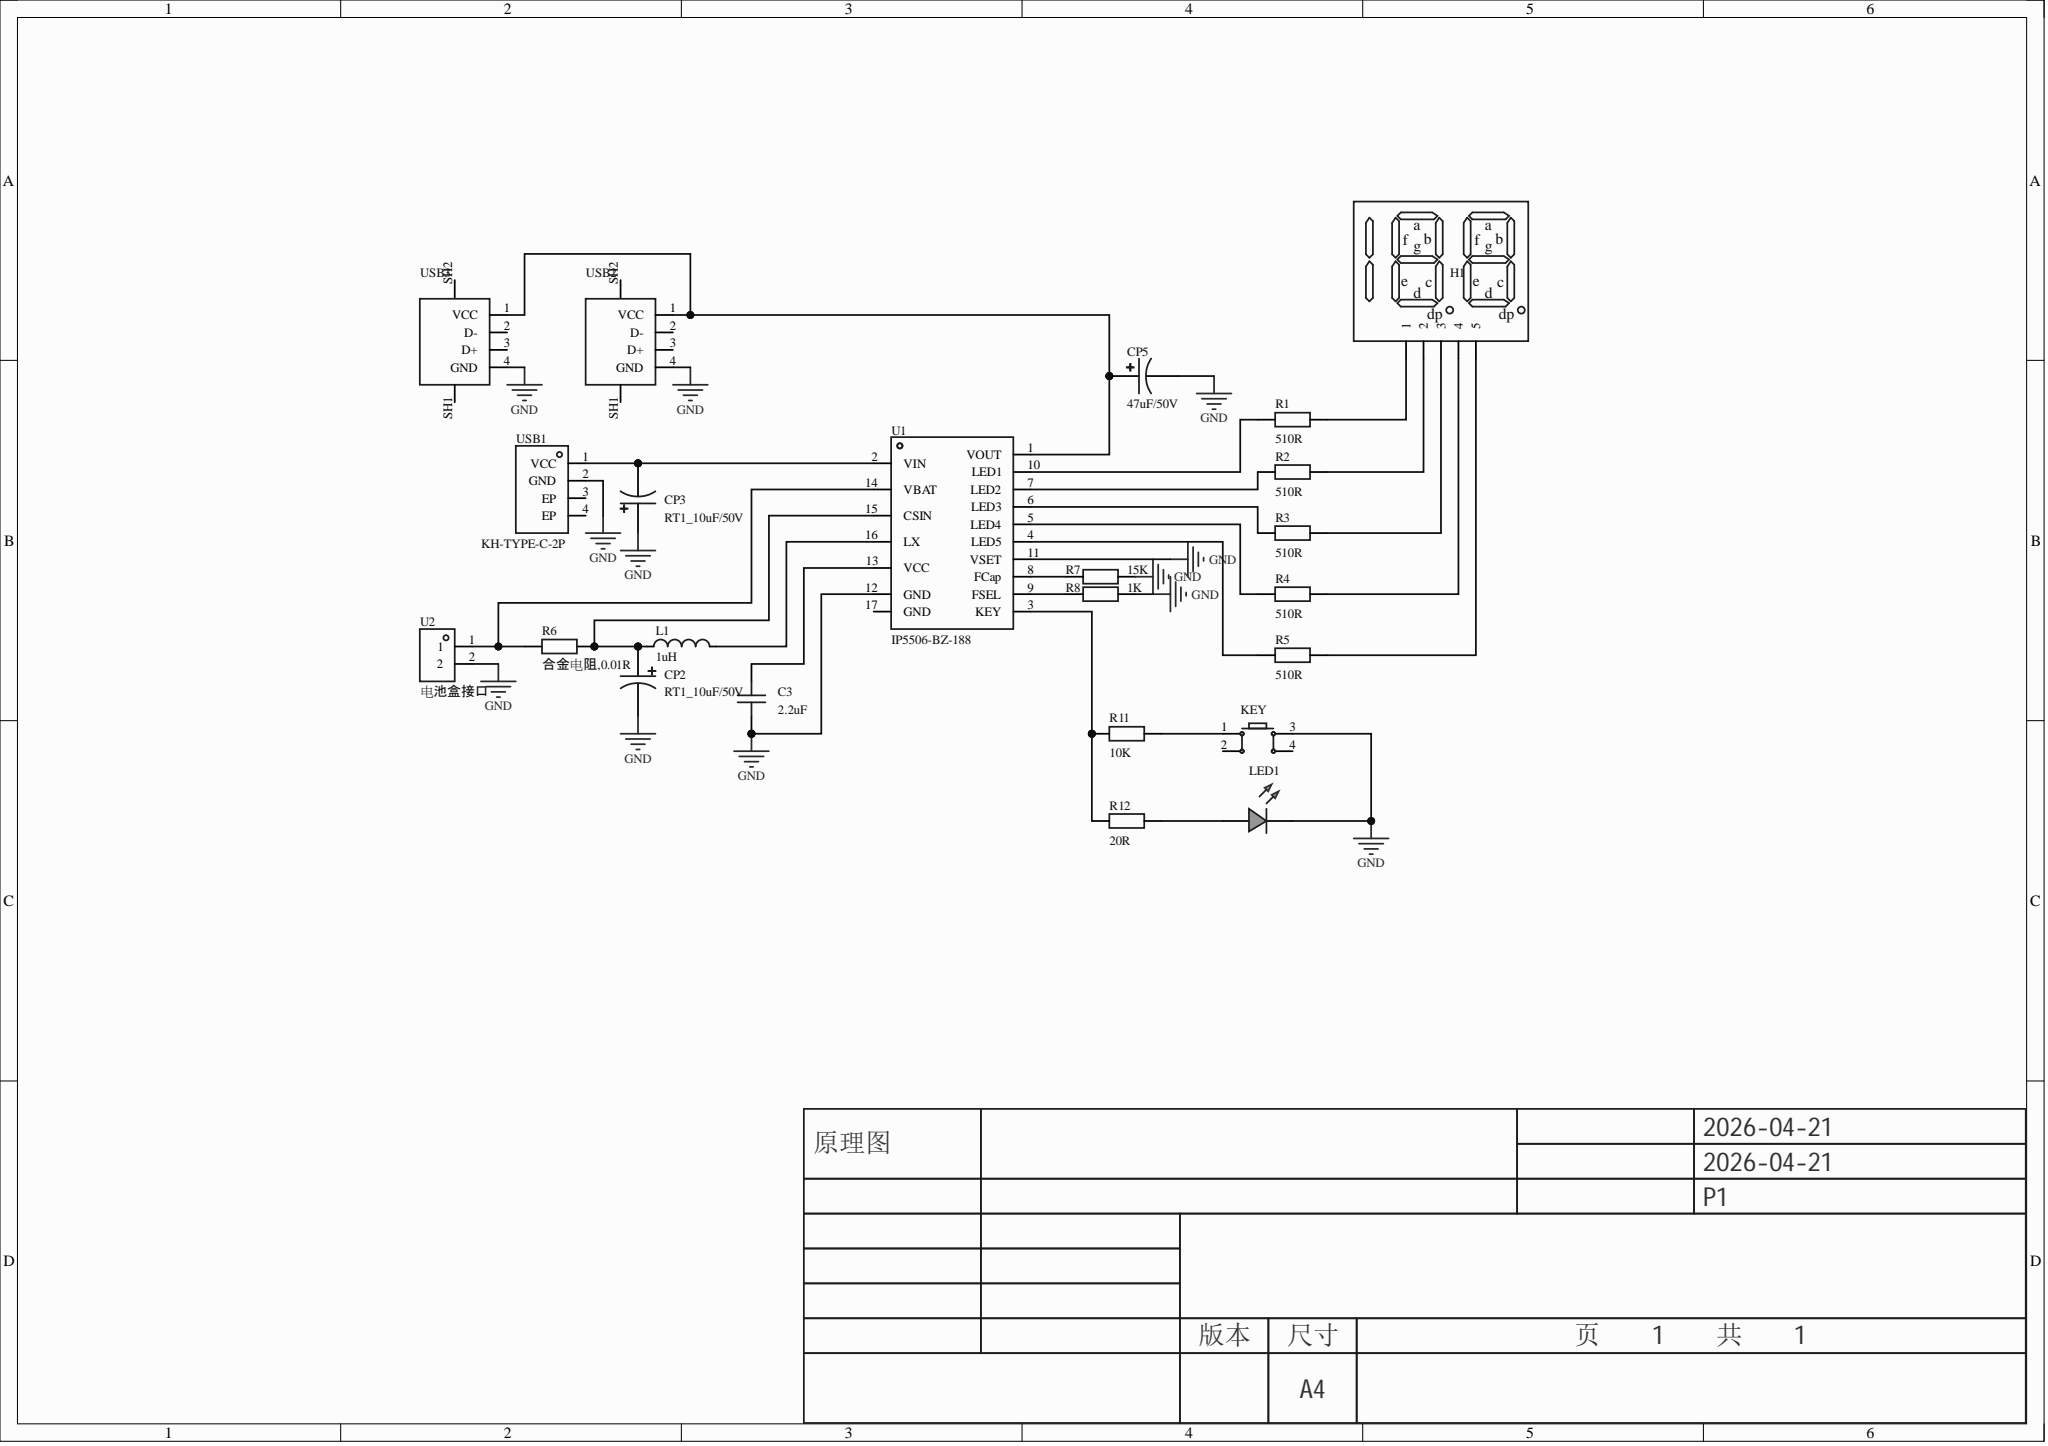Circuit board | Altium Designer | 23 parts | 22 nets
Bill of materials:
Comment,Description,Designator,Footprint,LibRef,Quantity
"2.2uF","","C3","C0805","CAP_0805","1"
"RT1_10uF/50V","","CP2, CP3","CAP-TH_BD5.0-P2.00-D0.8-FD","RT1_10uF/50V","2"
"47uF/50V","","CP5","CAP-SMD_BD6.3-L6.6-W6.6-LS7.0-FD","47uF/50V","1"
"","","H1","HDR-TH_5P-P2.54-V-F","HDR-F_2.54_1x5P","1"
"","","KEY","SW-TH_4P-L6.0-W6.0-P4.50-LS6.5","Key_TH_6x6x6","1"
"1uH","电感值:1uH;精度:±20%;饱和电流(Isat):15A;","L1","IND-SMD_L7.0-W6.6","SPM70701R0MESL","1"
"","","LED1","LED-TH_5mm","LED_TH-G_5mm","1"
"510R","","R1, R2, R3, R4, R5","R0805","Res_0805","5"
"合金电阻,0.01R","","R6","R1206","合金电阻,0.1R,+/-1%,R1206,1W.","1"
"15K","","R7","R0805","Res_0805","1"
"1K","","R8","R0805","Res_0805","1"
"10K","","R11","R0805","Res_0805","1"
"20R","","R12","R0805","Res_0805","1"
"IP5506-BZ-188","","U1","ESOP-16_L9.9-W3.9-P1.27-LS6.0-BL-EP","IP5506-BZ-188","1"
"电池盒接口","","U2","TH_C9900019910","电池盒接口","1"
"KH-TYPE-C-2P","连接器类型:Type-C;协议标准:-;公母:-;安装方式:弯插;触点数量:2P;端口数量:1;额定电流 - 电源:3A;工作温度:-25℃~+85℃;","USB1","USB-SMD_KH-TYPE-C-2P","KH-TYPE-C-2P","1"
"","","USB2, USB3","USB_ Type-A","USB_ Type-A","2"
Netlist (Protel format):
[
C3
C0805
2.2uF



]
[
CP2
CAP-TH_BD5.0-P2.00-D0.8-FD
RT1_10uF/50V



]
[
CP3
CAP-TH_BD5.0-P2.00-D0.8-FD
RT1_10uF/50V



]
[
CP5
CAP-SMD_BD6.3-L6.6-W6.6-LS7.0-FD
47uF/50V



]
[
H1
HDR-TH_5P-P2.54-V-F




]
[
KEY
SW-TH_4P-L6.0-W6.0-P4.50-LS6.5




]
[
L1
IND-SMD_L7.0-W6.6
1uH



]
[
LED1
LED-TH_5mm




]
[
R1
R0805
510R



]
[
R2
R0805
510R



]
[
R3
R0805
510R



]
[
R4
R0805
510R



]
[
R5
R0805
510R



]
[
R6
R1206
合金电阻,0.01R



]
[
R7
R0805
15K



]
[
R8
R0805
1K



]
[
R11
R0805
10K



]
[
R12
R0805
20R



]
[
U1
ESOP-16_L9.9-W3.9-P1.27-LS6.0-BL-EP
IP5506-BZ-188



]
[
U2
TH_C9900019910
电池盒接口



]
[
USB1
USB-SMD_KH-TYPE-C-2P
KH-TYPE-C-2P



]
[
USB2
USB_ Type-A




]
[
USB3
USB_ Type-A




]
(
NetR11_1
R11-1
R12-1
U1-3
)
(
NetR8_1
R8-1
U1-9
)
(
NetR7_1
R7-1
U1-8
)
(
NetR6_1
R6-1
U1-14
U2-1
)
(
NetR5_1
R5-1
U1-4
)
(
NetR4_1
R4-1
U1-5
)
(
NetR3_1
R3-1
U1-6
)
(
NetR2_1
R2-1
U1-7
)
(
NetR1_1
R1-1
U1-10
)
(
NetLED1_1
LED1-1
R12-2
)
(
NetL1_2
L1-2
U1-16
)
(
NetKEY_1
KEY-1
R11-2
)
(
NetH1_5
H1-5
R5-2
)
(
NetH1_4
H1-4
R4-2
)
(
NetH1_3
H1-3
R3-2
)
(
NetH1_2
H1-2
R2-2
)
(
NetH1_1
H1-1
R1-2
)
(
NetCP5_1
CP5-1
U1-1
USB2-1
USB3-1
)
(
NetCP3_2
CP3-2
U1-2
USB1-1
)
(
NetCP2_1
CP2-1
L1-1
R6-2
U1-15
)
(
NetC3_2
C3-2
U1-13
)
(
GND
C3-1
CP2-2
CP3-1
CP5-2
KEY-3
LED1-2
R7-2
R8-2
U1-11
U1-12
U2-2
USB1-2
USB2-4
USB3-4
)